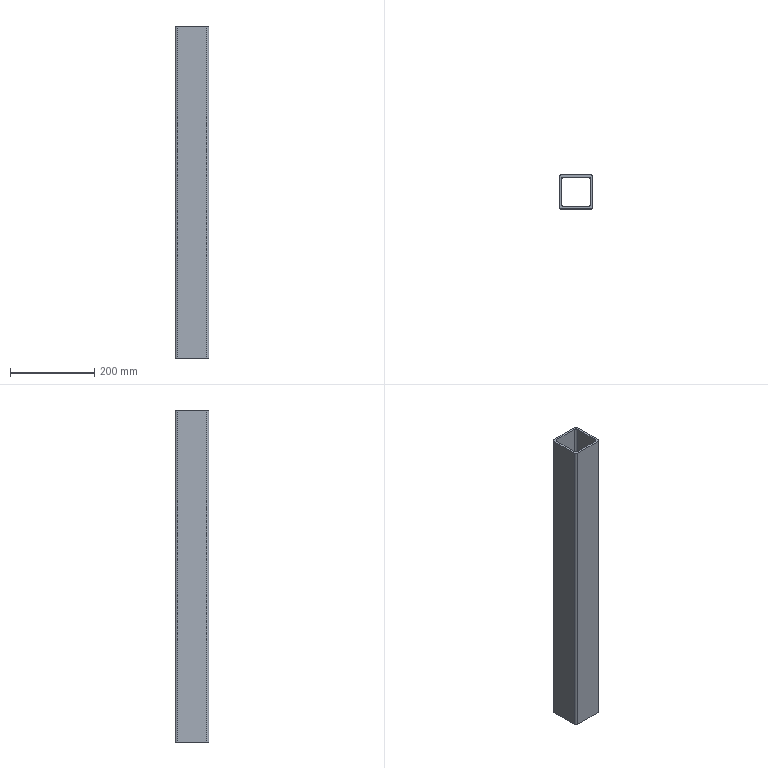Part | SolidWorks | features BaseBody 1 | 1 solid | 18 faces | box 80 x 80 x 790 mm | volume 1185000 mm3 | plane 10 | cylinder 8 | commonest cylinder face diameters 10 x8
STEP:
#1=CARTESIAN_POINT('',(40.,35.,395.));
#2=VERTEX_POINT('',#1);
#3=CARTESIAN_POINT('',(35.,40.,395.));
#4=VERTEX_POINT('',#3);
#5=CARTESIAN_POINT('',(35.,35.,395.));
#6=DIRECTION('',(0.,0.,1.));
#7=DIRECTION('',(1.,0.,0.));
#8=AXIS2_PLACEMENT_3D('',#5,#6,#7);
#9=CIRCLE('',#8,5.);
#10=EDGE_CURVE('',#2,#4,#9,.T.);
#11=ORIENTED_EDGE('',*,*,#10,.T.);
#12=CARTESIAN_POINT('',(-35.,40.,395.));
#13=VERTEX_POINT('',#12);
#14=CARTESIAN_POINT('',(35.,40.,395.));
#15=DIRECTION('',(-1.,0.,0.));
#16=VECTOR('',#15,1000.);
#17=LINE('',#14,#16);
#18=EDGE_CURVE('',#4,#13,#17,.T.);
#19=ORIENTED_EDGE('',*,*,#18,.T.);
#20=CARTESIAN_POINT('',(-40.,35.,395.));
#21=VERTEX_POINT('',#20);
#22=CARTESIAN_POINT('',(-35.,35.,395.));
#23=DIRECTION('',(0.,0.,1.));
#24=DIRECTION('',(1.,0.,0.));
#25=AXIS2_PLACEMENT_3D('',#22,#23,#24);
#26=CIRCLE('',#25,5.);
#27=EDGE_CURVE('',#13,#21,#26,.T.);
#28=ORIENTED_EDGE('',*,*,#27,.T.);
#29=CARTESIAN_POINT('',(-40.,-35.,395.));
#30=VERTEX_POINT('',#29);
#31=CARTESIAN_POINT('',(-40.,-35.,395.));
#32=DIRECTION('',(0.,-1.,0.));
#33=VECTOR('',#32,1000.);
#34=LINE('',#31,#33);
#35=EDGE_CURVE('',#21,#30,#34,.T.);
#36=ORIENTED_EDGE('',*,*,#35,.T.);
#37=CARTESIAN_POINT('',(-35.,-40.,395.));
#38=VERTEX_POINT('',#37);
#39=CARTESIAN_POINT('',(-35.,-35.,395.));
#40=DIRECTION('',(0.,0.,1.));
#41=DIRECTION('',(-1.,0.,0.));
#42=AXIS2_PLACEMENT_3D('',#39,#40,#41);
#43=CIRCLE('',#42,5.);
#44=EDGE_CURVE('',#30,#38,#43,.T.);
#45=ORIENTED_EDGE('',*,*,#44,.T.);
#46=CARTESIAN_POINT('',(35.,-40.,395.));
#47=VERTEX_POINT('',#46);
#48=CARTESIAN_POINT('',(35.,-40.,395.));
#49=DIRECTION('',(1.,0.,0.));
#50=VECTOR('',#49,1000.);
#51=LINE('',#48,#50);
#52=EDGE_CURVE('',#38,#47,#51,.T.);
#53=ORIENTED_EDGE('',*,*,#52,.T.);
#54=CARTESIAN_POINT('',(40.,-35.,395.));
#55=VERTEX_POINT('',#54);
#56=CARTESIAN_POINT('',(35.,-35.,395.));
#57=DIRECTION('',(0.,0.,1.));
#58=DIRECTION('',(1.,0.,0.));
#59=AXIS2_PLACEMENT_3D('',#56,#57,#58);
#60=CIRCLE('',#59,5.);
#61=EDGE_CURVE('',#47,#55,#60,.T.);
#62=ORIENTED_EDGE('',*,*,#61,.T.);
#63=CARTESIAN_POINT('',(40.,-35.,395.));
#64=DIRECTION('',(0.,1.,0.));
#65=VECTOR('',#64,1000.);
#66=LINE('',#63,#65);
#67=EDGE_CURVE('',#55,#2,#66,.T.);
#68=ORIENTED_EDGE('',*,*,#67,.T.);
#69=EDGE_LOOP('',(#11,#19,#28,#36,#45,#53,#62,#68));
#70=FACE_OUTER_BOUND('',#69,.T.);
#71=CARTESIAN_POINT('',(30.,35.,395.));
#72=VERTEX_POINT('',#71);
#73=CARTESIAN_POINT('',(-30.,35.,395.));
#74=VERTEX_POINT('',#73);
#75=CARTESIAN_POINT('',(30.,35.,395.));
#76=DIRECTION('',(-1.,0.,0.));
#77=VECTOR('',#76,1000.);
#78=LINE('',#75,#77);
#79=EDGE_CURVE('',#72,#74,#78,.T.);
#80=ORIENTED_EDGE('',*,*,#79,.F.);
#81=CARTESIAN_POINT('',(35.,30.,395.));
#82=VERTEX_POINT('',#81);
#83=CARTESIAN_POINT('',(30.,30.,395.));
#84=DIRECTION('',(0.,0.,1.));
#85=DIRECTION('',(1.,0.,0.));
#86=AXIS2_PLACEMENT_3D('',#83,#84,#85);
#87=CIRCLE('',#86,5.);
#88=EDGE_CURVE('',#82,#72,#87,.T.);
#89=ORIENTED_EDGE('',*,*,#88,.F.);
#90=CARTESIAN_POINT('',(35.,-30.,395.));
#91=VERTEX_POINT('',#90);
#92=CARTESIAN_POINT('',(35.,-30.,395.));
#93=DIRECTION('',(0.,1.,0.));
#94=VECTOR('',#93,1000.);
#95=LINE('',#92,#94);
#96=EDGE_CURVE('',#91,#82,#95,.T.);
#97=ORIENTED_EDGE('',*,*,#96,.F.);
#98=CARTESIAN_POINT('',(30.,-35.,395.));
#99=VERTEX_POINT('',#98);
#100=CARTESIAN_POINT('',(30.,-30.,395.));
#101=DIRECTION('',(0.,0.,1.));
#102=DIRECTION('',(1.,0.,0.));
#103=AXIS2_PLACEMENT_3D('',#100,#101,#102);
#104=CIRCLE('',#103,5.);
#105=EDGE_CURVE('',#99,#91,#104,.T.);
#106=ORIENTED_EDGE('',*,*,#105,.F.);
#107=CARTESIAN_POINT('',(-30.,-35.,395.));
#108=VERTEX_POINT('',#107);
#109=CARTESIAN_POINT('',(30.,-35.,395.));
#110=DIRECTION('',(1.,0.,0.));
#111=VECTOR('',#110,1000.);
#112=LINE('',#109,#111);
#113=EDGE_CURVE('',#108,#99,#112,.T.);
#114=ORIENTED_EDGE('',*,*,#113,.F.);
#115=CARTESIAN_POINT('',(-35.,-30.,395.));
#116=VERTEX_POINT('',#115);
#117=CARTESIAN_POINT('',(-30.,-30.,395.));
#118=DIRECTION('',(0.,0.,1.));
#119=DIRECTION('',(-1.,0.,0.));
#120=AXIS2_PLACEMENT_3D('',#117,#118,#119);
#121=CIRCLE('',#120,5.);
#122=EDGE_CURVE('',#116,#108,#121,.T.);
#123=ORIENTED_EDGE('',*,*,#122,.F.);
#124=CARTESIAN_POINT('',(-35.,30.,395.));
#125=VERTEX_POINT('',#124);
#126=CARTESIAN_POINT('',(-35.,-30.,395.));
#127=DIRECTION('',(0.,-1.,0.));
#128=VECTOR('',#127,1000.);
#129=LINE('',#126,#128);
#130=EDGE_CURVE('',#125,#116,#129,.T.);
#131=ORIENTED_EDGE('',*,*,#130,.F.);
#132=CARTESIAN_POINT('',(-30.,30.,395.));
#133=DIRECTION('',(0.,0.,1.));
#134=DIRECTION('',(1.,0.,0.));
#135=AXIS2_PLACEMENT_3D('',#132,#133,#134);
#136=CIRCLE('',#135,5.);
#137=EDGE_CURVE('',#74,#125,#136,.T.);
#138=ORIENTED_EDGE('',*,*,#137,.F.);
#139=EDGE_LOOP('',(#80,#89,#97,#106,#114,#123,#131,#138));
#140=FACE_BOUND('',#139,.T.);
#141=CARTESIAN_POINT('',(35.,35.,395.));
#142=DIRECTION('',(0.,0.,1.));
#143=DIRECTION('',(1.,0.,0.));
#144=AXIS2_PLACEMENT_3D('',#141,#142,#143);
#145=PLANE('',#144);
#146=ADVANCED_FACE('',(#70,#140),#145,.T.);
#147=CARTESIAN_POINT('',(40.,35.,-395.));
#148=VERTEX_POINT('',#147);
#149=CARTESIAN_POINT('',(35.,40.,-395.));
#150=VERTEX_POINT('',#149);
#151=CARTESIAN_POINT('',(35.,35.,-395.));
#152=DIRECTION('',(0.,0.,1.));
#153=DIRECTION('',(1.,0.,0.));
#154=AXIS2_PLACEMENT_3D('',#151,#152,#153);
#155=CIRCLE('',#154,5.);
#156=EDGE_CURVE('',#148,#150,#155,.T.);
#157=ORIENTED_EDGE('',*,*,#156,.F.);
#158=CARTESIAN_POINT('',(40.,-35.,-395.));
#159=VERTEX_POINT('',#158);
#160=CARTESIAN_POINT('',(40.,-35.,-395.));
#161=DIRECTION('',(0.,1.,0.));
#162=VECTOR('',#161,1000.);
#163=LINE('',#160,#162);
#164=EDGE_CURVE('',#159,#148,#163,.T.);
#165=ORIENTED_EDGE('',*,*,#164,.F.);
#166=CARTESIAN_POINT('',(35.,-40.,-395.));
#167=VERTEX_POINT('',#166);
#168=CARTESIAN_POINT('',(35.,-35.,-395.));
#169=DIRECTION('',(0.,0.,1.));
#170=DIRECTION('',(1.,0.,0.));
#171=AXIS2_PLACEMENT_3D('',#168,#169,#170);
#172=CIRCLE('',#171,5.);
#173=EDGE_CURVE('',#167,#159,#172,.T.);
#174=ORIENTED_EDGE('',*,*,#173,.F.);
#175=CARTESIAN_POINT('',(-35.,-40.,-395.));
#176=VERTEX_POINT('',#175);
#177=CARTESIAN_POINT('',(35.,-40.,-395.));
#178=DIRECTION('',(1.,0.,0.));
#179=VECTOR('',#178,1000.);
#180=LINE('',#177,#179);
#181=EDGE_CURVE('',#176,#167,#180,.T.);
#182=ORIENTED_EDGE('',*,*,#181,.F.);
#183=CARTESIAN_POINT('',(-40.,-35.,-395.));
#184=VERTEX_POINT('',#183);
#185=CARTESIAN_POINT('',(-35.,-35.,-395.));
#186=DIRECTION('',(0.,0.,1.));
#187=DIRECTION('',(-1.,0.,0.));
#188=AXIS2_PLACEMENT_3D('',#185,#186,#187);
#189=CIRCLE('',#188,5.);
#190=EDGE_CURVE('',#184,#176,#189,.T.);
#191=ORIENTED_EDGE('',*,*,#190,.F.);
#192=CARTESIAN_POINT('',(-40.,35.,-395.));
#193=VERTEX_POINT('',#192);
#194=CARTESIAN_POINT('',(-40.,-35.,-395.));
#195=DIRECTION('',(0.,-1.,0.));
#196=VECTOR('',#195,1000.);
#197=LINE('',#194,#196);
#198=EDGE_CURVE('',#193,#184,#197,.T.);
#199=ORIENTED_EDGE('',*,*,#198,.F.);
#200=CARTESIAN_POINT('',(-35.,40.,-395.));
#201=VERTEX_POINT('',#200);
#202=CARTESIAN_POINT('',(-35.,35.,-395.));
#203=DIRECTION('',(0.,0.,1.));
#204=DIRECTION('',(1.,0.,0.));
#205=AXIS2_PLACEMENT_3D('',#202,#203,#204);
#206=CIRCLE('',#205,5.);
#207=EDGE_CURVE('',#201,#193,#206,.T.);
#208=ORIENTED_EDGE('',*,*,#207,.F.);
#209=CARTESIAN_POINT('',(35.,40.,-395.));
#210=DIRECTION('',(-1.,0.,0.));
#211=VECTOR('',#210,1000.);
#212=LINE('',#209,#211);
#213=EDGE_CURVE('',#150,#201,#212,.T.);
#214=ORIENTED_EDGE('',*,*,#213,.F.);
#215=EDGE_LOOP('',(#157,#165,#174,#182,#191,#199,#208,#214));
#216=FACE_OUTER_BOUND('',#215,.T.);
#217=CARTESIAN_POINT('',(35.,30.,-395.));
#218=VERTEX_POINT('',#217);
#219=CARTESIAN_POINT('',(30.,35.,-395.));
#220=VERTEX_POINT('',#219);
#221=CARTESIAN_POINT('',(30.,30.,-395.));
#222=DIRECTION('',(0.,0.,1.));
#223=DIRECTION('',(1.,0.,0.));
#224=AXIS2_PLACEMENT_3D('',#221,#222,#223);
#225=CIRCLE('',#224,5.);
#226=EDGE_CURVE('',#218,#220,#225,.T.);
#227=ORIENTED_EDGE('',*,*,#226,.T.);
#228=CARTESIAN_POINT('',(-30.,35.,-395.));
#229=VERTEX_POINT('',#228);
#230=CARTESIAN_POINT('',(30.,35.,-395.));
#231=DIRECTION('',(-1.,0.,0.));
#232=VECTOR('',#231,1000.);
#233=LINE('',#230,#232);
#234=EDGE_CURVE('',#220,#229,#233,.T.);
#235=ORIENTED_EDGE('',*,*,#234,.T.);
#236=CARTESIAN_POINT('',(-35.,30.,-395.));
#237=VERTEX_POINT('',#236);
#238=CARTESIAN_POINT('',(-30.,30.,-395.));
#239=DIRECTION('',(0.,0.,1.));
#240=DIRECTION('',(1.,0.,0.));
#241=AXIS2_PLACEMENT_3D('',#238,#239,#240);
#242=CIRCLE('',#241,5.);
#243=EDGE_CURVE('',#229,#237,#242,.T.);
#244=ORIENTED_EDGE('',*,*,#243,.T.);
#245=CARTESIAN_POINT('',(-35.,-30.,-395.));
#246=VERTEX_POINT('',#245);
#247=CARTESIAN_POINT('',(-35.,-30.,-395.));
#248=DIRECTION('',(0.,-1.,0.));
#249=VECTOR('',#248,1000.);
#250=LINE('',#247,#249);
#251=EDGE_CURVE('',#237,#246,#250,.T.);
#252=ORIENTED_EDGE('',*,*,#251,.T.);
#253=CARTESIAN_POINT('',(-30.,-35.,-395.));
#254=VERTEX_POINT('',#253);
#255=CARTESIAN_POINT('',(-30.,-30.,-395.));
#256=DIRECTION('',(0.,0.,1.));
#257=DIRECTION('',(-1.,0.,0.));
#258=AXIS2_PLACEMENT_3D('',#255,#256,#257);
#259=CIRCLE('',#258,5.);
#260=EDGE_CURVE('',#246,#254,#259,.T.);
#261=ORIENTED_EDGE('',*,*,#260,.T.);
#262=CARTESIAN_POINT('',(30.,-35.,-395.));
#263=VERTEX_POINT('',#262);
#264=CARTESIAN_POINT('',(30.,-35.,-395.));
#265=DIRECTION('',(1.,0.,0.));
#266=VECTOR('',#265,1000.);
#267=LINE('',#264,#266);
#268=EDGE_CURVE('',#254,#263,#267,.T.);
#269=ORIENTED_EDGE('',*,*,#268,.T.);
#270=CARTESIAN_POINT('',(35.,-30.,-395.));
#271=VERTEX_POINT('',#270);
#272=CARTESIAN_POINT('',(30.,-30.,-395.));
#273=DIRECTION('',(0.,0.,1.));
#274=DIRECTION('',(1.,0.,0.));
#275=AXIS2_PLACEMENT_3D('',#272,#273,#274);
#276=CIRCLE('',#275,5.);
#277=EDGE_CURVE('',#263,#271,#276,.T.);
#278=ORIENTED_EDGE('',*,*,#277,.T.);
#279=CARTESIAN_POINT('',(35.,-30.,-395.));
#280=DIRECTION('',(0.,1.,0.));
#281=VECTOR('',#280,1000.);
#282=LINE('',#279,#281);
#283=EDGE_CURVE('',#271,#218,#282,.T.);
#284=ORIENTED_EDGE('',*,*,#283,.T.);
#285=EDGE_LOOP('',(#227,#235,#244,#252,#261,#269,#278,#284));
#286=FACE_BOUND('',#285,.T.);
#287=CARTESIAN_POINT('',(35.,35.,-395.));
#288=DIRECTION('',(0.,0.,1.));
#289=DIRECTION('',(1.,0.,0.));
#290=AXIS2_PLACEMENT_3D('',#287,#288,#289);
#291=PLANE('',#290);
#292=ADVANCED_FACE('',(#216,#286),#291,.F.);
#293=ORIENTED_EDGE('',*,*,#156,.T.);
#294=CARTESIAN_POINT('',(35.,40.,395.));
#295=DIRECTION('',(0.,0.,-1.));
#296=VECTOR('',#295,1000.);
#297=LINE('',#294,#296);
#298=EDGE_CURVE('',#4,#150,#297,.T.);
#299=ORIENTED_EDGE('',*,*,#298,.F.);
#300=ORIENTED_EDGE('',*,*,#10,.F.);
#301=CARTESIAN_POINT('',(40.,35.,395.));
#302=DIRECTION('',(0.,0.,-1.));
#303=VECTOR('',#302,1000.);
#304=LINE('',#301,#303);
#305=EDGE_CURVE('',#2,#148,#304,.T.);
#306=ORIENTED_EDGE('',*,*,#305,.T.);
#307=EDGE_LOOP('',(#293,#299,#300,#306));
#308=FACE_OUTER_BOUND('',#307,.T.);
#309=CARTESIAN_POINT('',(35.,35.,395.));
#310=DIRECTION('',(0.,0.,-1.));
#311=DIRECTION('',(-1.,0.,0.));
#312=AXIS2_PLACEMENT_3D('',#309,#310,#311);
#313=CYLINDRICAL_SURFACE('',#312,5.);
#314=ADVANCED_FACE('',(#308),#313,.T.);
#315=ORIENTED_EDGE('',*,*,#213,.T.);
#316=CARTESIAN_POINT('',(-35.,40.,395.));
#317=DIRECTION('',(0.,0.,-1.));
#318=VECTOR('',#317,1000.);
#319=LINE('',#316,#318);
#320=EDGE_CURVE('',#13,#201,#319,.T.);
#321=ORIENTED_EDGE('',*,*,#320,.F.);
#322=ORIENTED_EDGE('',*,*,#18,.F.);
#323=ORIENTED_EDGE('',*,*,#298,.T.);
#324=EDGE_LOOP('',(#315,#321,#322,#323));
#325=FACE_OUTER_BOUND('',#324,.T.);
#326=CARTESIAN_POINT('',(35.,40.,395.));
#327=DIRECTION('',(0.,-1.,0.));
#328=DIRECTION('',(0.,0.,-1.));
#329=AXIS2_PLACEMENT_3D('',#326,#327,#328);
#330=PLANE('',#329);
#331=ADVANCED_FACE('',(#325),#330,.F.);
#332=ORIENTED_EDGE('',*,*,#207,.T.);
#333=CARTESIAN_POINT('',(-40.,35.,395.));
#334=DIRECTION('',(0.,0.,-1.));
#335=VECTOR('',#334,1000.);
#336=LINE('',#333,#335);
#337=EDGE_CURVE('',#21,#193,#336,.T.);
#338=ORIENTED_EDGE('',*,*,#337,.F.);
#339=ORIENTED_EDGE('',*,*,#27,.F.);
#340=ORIENTED_EDGE('',*,*,#320,.T.);
#341=EDGE_LOOP('',(#332,#338,#339,#340));
#342=FACE_OUTER_BOUND('',#341,.T.);
#343=CARTESIAN_POINT('',(-35.,35.,395.));
#344=DIRECTION('',(0.,0.,-1.));
#345=DIRECTION('',(-1.,0.,0.));
#346=AXIS2_PLACEMENT_3D('',#343,#344,#345);
#347=CYLINDRICAL_SURFACE('',#346,5.);
#348=ADVANCED_FACE('',(#342),#347,.T.);
#349=ORIENTED_EDGE('',*,*,#198,.T.);
#350=CARTESIAN_POINT('',(-40.,-35.,395.));
#351=DIRECTION('',(0.,0.,-1.));
#352=VECTOR('',#351,1000.);
#353=LINE('',#350,#352);
#354=EDGE_CURVE('',#30,#184,#353,.T.);
#355=ORIENTED_EDGE('',*,*,#354,.F.);
#356=ORIENTED_EDGE('',*,*,#35,.F.);
#357=ORIENTED_EDGE('',*,*,#337,.T.);
#358=EDGE_LOOP('',(#349,#355,#356,#357));
#359=FACE_OUTER_BOUND('',#358,.T.);
#360=CARTESIAN_POINT('',(-40.,-35.,395.));
#361=DIRECTION('',(1.,0.,0.));
#362=DIRECTION('',(0.,0.,-1.));
#363=AXIS2_PLACEMENT_3D('',#360,#361,#362);
#364=PLANE('',#363);
#365=ADVANCED_FACE('',(#359),#364,.F.);
#366=ORIENTED_EDGE('',*,*,#190,.T.);
#367=CARTESIAN_POINT('',(-35.,-40.,395.));
#368=DIRECTION('',(0.,0.,-1.));
#369=VECTOR('',#368,1000.);
#370=LINE('',#367,#369);
#371=EDGE_CURVE('',#38,#176,#370,.T.);
#372=ORIENTED_EDGE('',*,*,#371,.F.);
#373=ORIENTED_EDGE('',*,*,#44,.F.);
#374=ORIENTED_EDGE('',*,*,#354,.T.);
#375=EDGE_LOOP('',(#366,#372,#373,#374));
#376=FACE_OUTER_BOUND('',#375,.T.);
#377=CARTESIAN_POINT('',(-35.,-35.,395.));
#378=DIRECTION('',(0.,0.,-1.));
#379=DIRECTION('',(-1.,0.,0.));
#380=AXIS2_PLACEMENT_3D('',#377,#378,#379);
#381=CYLINDRICAL_SURFACE('',#380,5.);
#382=ADVANCED_FACE('',(#376),#381,.T.);
#383=ORIENTED_EDGE('',*,*,#181,.T.);
#384=CARTESIAN_POINT('',(35.,-40.,395.));
#385=DIRECTION('',(0.,0.,-1.));
#386=VECTOR('',#385,1000.);
#387=LINE('',#384,#386);
#388=EDGE_CURVE('',#47,#167,#387,.T.);
#389=ORIENTED_EDGE('',*,*,#388,.F.);
#390=ORIENTED_EDGE('',*,*,#52,.F.);
#391=ORIENTED_EDGE('',*,*,#371,.T.);
#392=EDGE_LOOP('',(#383,#389,#390,#391));
#393=FACE_OUTER_BOUND('',#392,.T.);
#394=CARTESIAN_POINT('',(35.,-40.,395.));
#395=DIRECTION('',(0.,1.,0.));
#396=DIRECTION('',(-1.,0.,0.));
#397=AXIS2_PLACEMENT_3D('',#394,#395,#396);
#398=PLANE('',#397);
#399=ADVANCED_FACE('',(#393),#398,.F.);
#400=ORIENTED_EDGE('',*,*,#173,.T.);
#401=CARTESIAN_POINT('',(40.,-35.,395.));
#402=DIRECTION('',(0.,0.,-1.));
#403=VECTOR('',#402,1000.);
#404=LINE('',#401,#403);
#405=EDGE_CURVE('',#55,#159,#404,.T.);
#406=ORIENTED_EDGE('',*,*,#405,.F.);
#407=ORIENTED_EDGE('',*,*,#61,.F.);
#408=ORIENTED_EDGE('',*,*,#388,.T.);
#409=EDGE_LOOP('',(#400,#406,#407,#408));
#410=FACE_OUTER_BOUND('',#409,.T.);
#411=CARTESIAN_POINT('',(35.,-35.,395.));
#412=DIRECTION('',(0.,0.,-1.));
#413=DIRECTION('',(-1.,0.,0.));
#414=AXIS2_PLACEMENT_3D('',#411,#412,#413);
#415=CYLINDRICAL_SURFACE('',#414,5.);
#416=ADVANCED_FACE('',(#410),#415,.T.);
#417=ORIENTED_EDGE('',*,*,#164,.T.);
#418=ORIENTED_EDGE('',*,*,#305,.F.);
#419=ORIENTED_EDGE('',*,*,#67,.F.);
#420=ORIENTED_EDGE('',*,*,#405,.T.);
#421=EDGE_LOOP('',(#417,#418,#419,#420));
#422=FACE_OUTER_BOUND('',#421,.T.);
#423=CARTESIAN_POINT('',(40.,-35.,395.));
#424=DIRECTION('',(-1.,0.,0.));
#425=DIRECTION('',(0.,0.,1.));
#426=AXIS2_PLACEMENT_3D('',#423,#424,#425);
#427=PLANE('',#426);
#428=ADVANCED_FACE('',(#422),#427,.F.);
#429=ORIENTED_EDGE('',*,*,#226,.F.);
#430=CARTESIAN_POINT('',(35.,30.,395.));
#431=DIRECTION('',(0.,0.,-1.));
#432=VECTOR('',#431,1000.);
#433=LINE('',#430,#432);
#434=EDGE_CURVE('',#82,#218,#433,.T.);
#435=ORIENTED_EDGE('',*,*,#434,.F.);
#436=ORIENTED_EDGE('',*,*,#88,.T.);
#437=CARTESIAN_POINT('',(30.,35.,395.));
#438=DIRECTION('',(0.,0.,-1.));
#439=VECTOR('',#438,1000.);
#440=LINE('',#437,#439);
#441=EDGE_CURVE('',#72,#220,#440,.T.);
#442=ORIENTED_EDGE('',*,*,#441,.T.);
#443=EDGE_LOOP('',(#429,#435,#436,#442));
#444=FACE_OUTER_BOUND('',#443,.T.);
#445=CARTESIAN_POINT('',(30.,30.,395.));
#446=DIRECTION('',(0.,0.,-1.));
#447=DIRECTION('',(-1.,0.,0.));
#448=AXIS2_PLACEMENT_3D('',#445,#446,#447);
#449=CYLINDRICAL_SURFACE('',#448,5.);
#450=ADVANCED_FACE('',(#444),#449,.F.);
#451=ORIENTED_EDGE('',*,*,#234,.F.);
#452=ORIENTED_EDGE('',*,*,#441,.F.);
#453=ORIENTED_EDGE('',*,*,#79,.T.);
#454=CARTESIAN_POINT('',(-30.,35.,395.));
#455=DIRECTION('',(0.,0.,-1.));
#456=VECTOR('',#455,1000.);
#457=LINE('',#454,#456);
#458=EDGE_CURVE('',#74,#229,#457,.T.);
#459=ORIENTED_EDGE('',*,*,#458,.T.);
#460=EDGE_LOOP('',(#451,#452,#453,#459));
#461=FACE_OUTER_BOUND('',#460,.T.);
#462=CARTESIAN_POINT('',(30.,35.,395.));
#463=DIRECTION('',(0.,-1.,0.));
#464=DIRECTION('',(0.,0.,-1.));
#465=AXIS2_PLACEMENT_3D('',#462,#463,#464);
#466=PLANE('',#465);
#467=ADVANCED_FACE('',(#461),#466,.T.);
#468=ORIENTED_EDGE('',*,*,#243,.F.);
#469=ORIENTED_EDGE('',*,*,#458,.F.);
#470=ORIENTED_EDGE('',*,*,#137,.T.);
#471=CARTESIAN_POINT('',(-35.,30.,395.));
#472=DIRECTION('',(0.,0.,-1.));
#473=VECTOR('',#472,1000.);
#474=LINE('',#471,#473);
#475=EDGE_CURVE('',#125,#237,#474,.T.);
#476=ORIENTED_EDGE('',*,*,#475,.T.);
#477=EDGE_LOOP('',(#468,#469,#470,#476));
#478=FACE_OUTER_BOUND('',#477,.T.);
#479=CARTESIAN_POINT('',(-30.,30.,395.));
#480=DIRECTION('',(0.,0.,-1.));
#481=DIRECTION('',(-1.,0.,0.));
#482=AXIS2_PLACEMENT_3D('',#479,#480,#481);
#483=CYLINDRICAL_SURFACE('',#482,5.);
#484=ADVANCED_FACE('',(#478),#483,.F.);
#485=ORIENTED_EDGE('',*,*,#251,.F.);
#486=ORIENTED_EDGE('',*,*,#475,.F.);
#487=ORIENTED_EDGE('',*,*,#130,.T.);
#488=CARTESIAN_POINT('',(-35.,-30.,395.));
#489=DIRECTION('',(0.,0.,-1.));
#490=VECTOR('',#489,1000.);
#491=LINE('',#488,#490);
#492=EDGE_CURVE('',#116,#246,#491,.T.);
#493=ORIENTED_EDGE('',*,*,#492,.T.);
#494=EDGE_LOOP('',(#485,#486,#487,#493));
#495=FACE_OUTER_BOUND('',#494,.T.);
#496=CARTESIAN_POINT('',(-35.,-30.,395.));
#497=DIRECTION('',(1.,0.,0.));
#498=DIRECTION('',(0.,1.,0.));
#499=AXIS2_PLACEMENT_3D('',#496,#497,#498);
#500=PLANE('',#499);
#501=ADVANCED_FACE('',(#495),#500,.T.);
#502=ORIENTED_EDGE('',*,*,#260,.F.);
#503=ORIENTED_EDGE('',*,*,#492,.F.);
#504=ORIENTED_EDGE('',*,*,#122,.T.);
#505=CARTESIAN_POINT('',(-30.,-35.,395.));
#506=DIRECTION('',(0.,0.,-1.));
#507=VECTOR('',#506,1000.);
#508=LINE('',#505,#507);
#509=EDGE_CURVE('',#108,#254,#508,.T.);
#510=ORIENTED_EDGE('',*,*,#509,.T.);
#511=EDGE_LOOP('',(#502,#503,#504,#510));
#512=FACE_OUTER_BOUND('',#511,.T.);
#513=CARTESIAN_POINT('',(-30.,-30.,395.));
#514=DIRECTION('',(0.,0.,-1.));
#515=DIRECTION('',(-1.,0.,0.));
#516=AXIS2_PLACEMENT_3D('',#513,#514,#515);
#517=CYLINDRICAL_SURFACE('',#516,5.);
#518=ADVANCED_FACE('',(#512),#517,.F.);
#519=ORIENTED_EDGE('',*,*,#268,.F.);
#520=ORIENTED_EDGE('',*,*,#509,.F.);
#521=ORIENTED_EDGE('',*,*,#113,.T.);
#522=CARTESIAN_POINT('',(30.,-35.,395.));
#523=DIRECTION('',(0.,0.,-1.));
#524=VECTOR('',#523,1000.);
#525=LINE('',#522,#524);
#526=EDGE_CURVE('',#99,#263,#525,.T.);
#527=ORIENTED_EDGE('',*,*,#526,.T.);
#528=EDGE_LOOP('',(#519,#520,#521,#527));
#529=FACE_OUTER_BOUND('',#528,.T.);
#530=CARTESIAN_POINT('',(30.,-35.,395.));
#531=DIRECTION('',(0.,1.,0.));
#532=DIRECTION('',(-1.,0.,0.));
#533=AXIS2_PLACEMENT_3D('',#530,#531,#532);
#534=PLANE('',#533);
#535=ADVANCED_FACE('',(#529),#534,.T.);
#536=ORIENTED_EDGE('',*,*,#277,.F.);
#537=ORIENTED_EDGE('',*,*,#526,.F.);
#538=ORIENTED_EDGE('',*,*,#105,.T.);
#539=CARTESIAN_POINT('',(35.,-30.,395.));
#540=DIRECTION('',(0.,0.,-1.));
#541=VECTOR('',#540,1000.);
#542=LINE('',#539,#541);
#543=EDGE_CURVE('',#91,#271,#542,.T.);
#544=ORIENTED_EDGE('',*,*,#543,.T.);
#545=EDGE_LOOP('',(#536,#537,#538,#544));
#546=FACE_OUTER_BOUND('',#545,.T.);
#547=CARTESIAN_POINT('',(30.,-30.,395.));
#548=DIRECTION('',(0.,0.,-1.));
#549=DIRECTION('',(-1.,0.,0.));
#550=AXIS2_PLACEMENT_3D('',#547,#548,#549);
#551=CYLINDRICAL_SURFACE('',#550,5.);
#552=ADVANCED_FACE('',(#546),#551,.F.);
#553=ORIENTED_EDGE('',*,*,#283,.F.);
#554=ORIENTED_EDGE('',*,*,#543,.F.);
#555=ORIENTED_EDGE('',*,*,#96,.T.);
#556=ORIENTED_EDGE('',*,*,#434,.T.);
#557=EDGE_LOOP('',(#553,#554,#555,#556));
#558=FACE_OUTER_BOUND('',#557,.T.);
#559=CARTESIAN_POINT('',(35.,-30.,395.));
#560=DIRECTION('',(-1.,0.,0.));
#561=DIRECTION('',(0.,0.,1.));
#562=AXIS2_PLACEMENT_3D('',#559,#560,#561);
#563=PLANE('',#562);
#564=ADVANCED_FACE('',(#558),#563,.T.);
#565=CLOSED_SHELL('',(#146,#292,#314,#331,#348,#365,#382,#399,#416,#428,#450,#467,#484,#501,#518,#535,#552,#564));
#566=MANIFOLD_SOLID_BREP('',#565);
#567=CARTESIAN_POINT('',(0.,0.,0.));
#568=DIRECTION('',(0.,0.,1.));
#569=DIRECTION('',(1.,0.,0.));
#570=AXIS2_PLACEMENT_3D('',#567,#568,#569);
#571=(LENGTH_UNIT()NAMED_UNIT(*)SI_UNIT(.MILLI.,.METRE.));
#572=UNCERTAINTY_MEASURE_WITH_UNIT(LENGTH_MEASURE(0.00001),#571,'','');
#573=(NAMED_UNIT(*)PLANE_ANGLE_UNIT()SI_UNIT($,.RADIAN.));
#574=(NAMED_UNIT(*)SI_UNIT($,.STERADIAN.)SOLID_ANGLE_UNIT());
#575=(GEOMETRIC_REPRESENTATION_CONTEXT(3)GLOBAL_UNCERTAINTY_ASSIGNED_CONTEXT((#572))GLOBAL_UNIT_ASSIGNED_CONTEXT((#571,#573,#574))REPRESENTATION_CONTEXT('',''));
#576=ADVANCED_BREP_SHAPE_REPRESENTATION('',(#566,#570),#575);